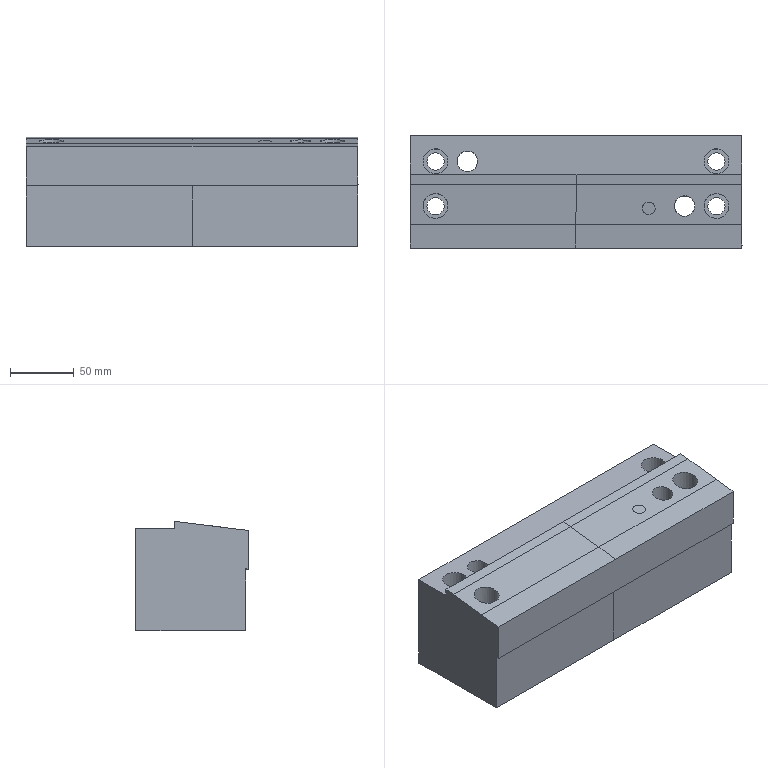Part | NX | features solid 2 | 1 solid | 31 faces | box 260 x 88.001 x 85.748 mm | volume 1716086 mm3 | spline 11 | plane 10 | cylinder 10 | commonest cylinder face diameters 13.5 x4 19.5 x4 16 x2